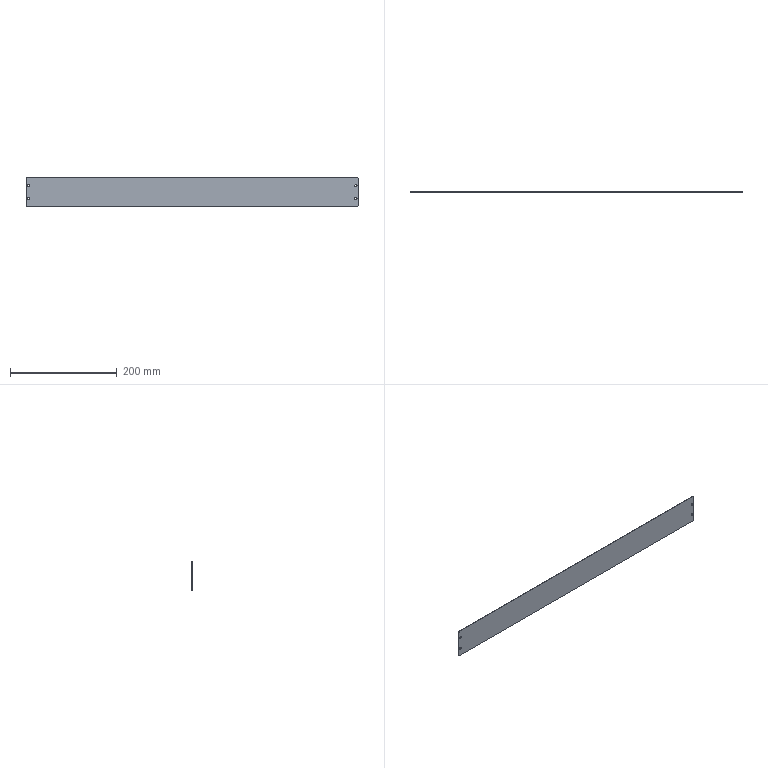Part | STEP file | ASND-0110-TCTF01-30(default)-1 | 1 solid | 22 faces | box 622 x 1.5 x 56 mm | volume 52147 mm3 | cylinder 16 | plane 6 | commonest cylinder face diameters 4 x8 4.5 x8